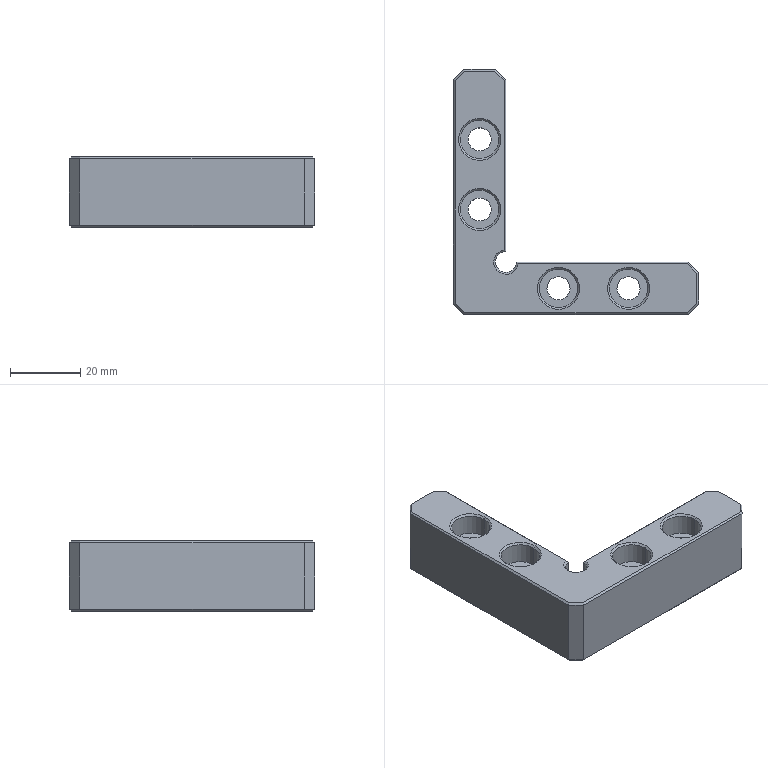Part | SolidWorks | features BaseBody 1 | 1 solid | 77 faces | box 70 x 70 x 20 mm | volume 32234 mm3 | plane 39 | cone 20 | cylinder 18 | commonest cylinder face diameters 6.6 x8 11 x8 6 x2